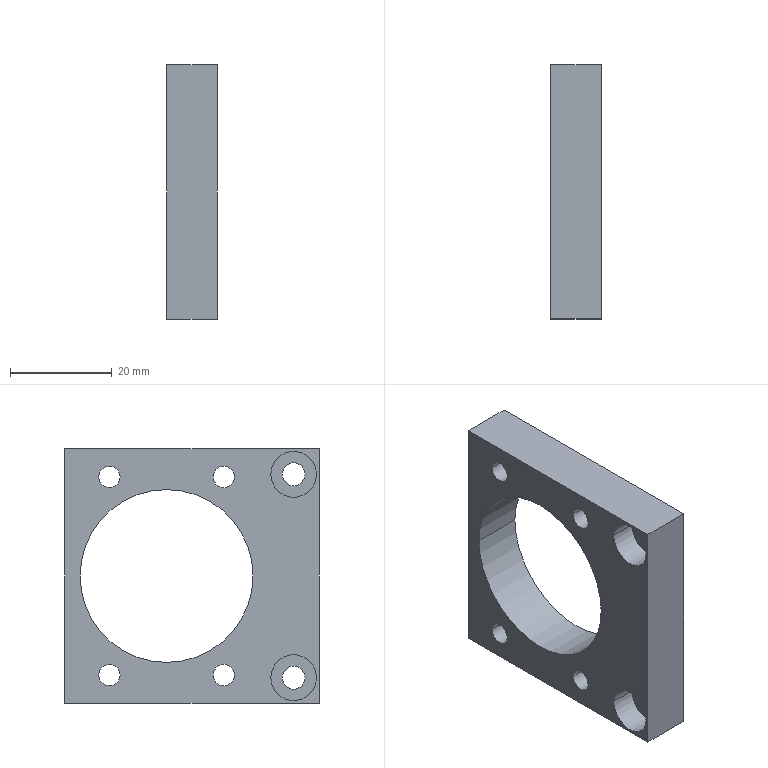Part | STEP file | 03-19 Lead screw head fixing plate 1 | 1 solid | 26 faces | box 10 x 50 x 50 mm | volume 14571 mm3 | cylinder 18 | plane 8 | commonest cylinder face diameters 4.2 x8 4.5 x4 9 x4 34 x2